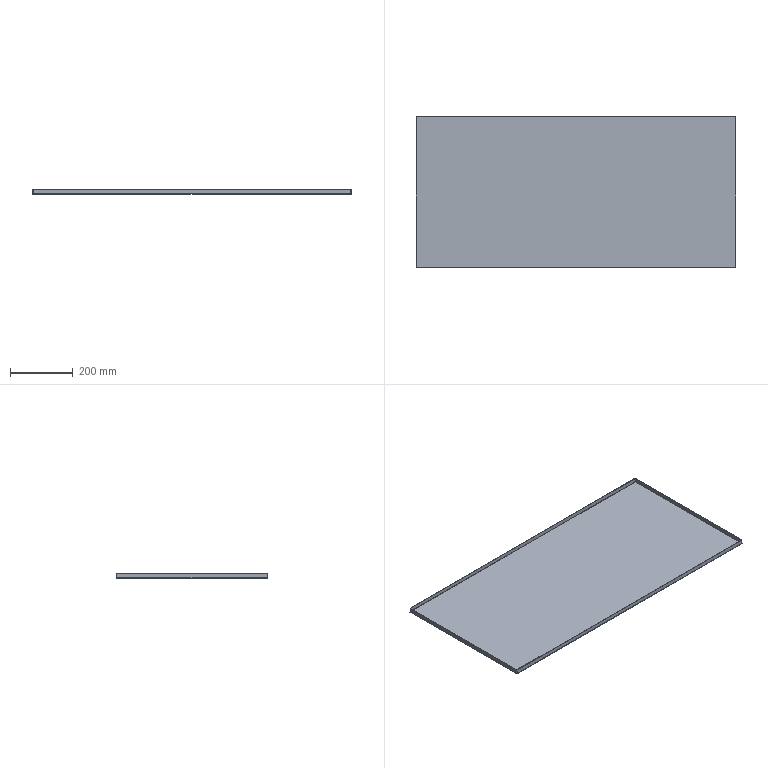Part | SolidWorks | 1 solid | 38 faces | box 1020 x 485 x 15 mm | volume 1064228 mm3 | plane 22 | spline 8 | cylinder 8 | commonest cylinder face diameters 0.2 x4 4.2 x4
STEP:
#1=CARTESIAN_POINT('',(507.9,-240.4,-2.));
#2=VERTEX_POINT('',#1);
#3=CARTESIAN_POINT('',(-507.9,-240.4,-2.));
#4=VERTEX_POINT('',#3);
#5=CARTESIAN_POINT('',(507.9,-240.4,-2.));
#6=DIRECTION('',(-1.,0.,0.));
#7=VECTOR('',#6,1000.);
#8=LINE('',#5,#7);
#9=EDGE_CURVE('',#2,#4,#8,.T.);
#10=ORIENTED_EDGE('',*,*,#9,.T.);
#11=CARTESIAN_POINT('',(-507.9,240.4,-2.));
#12=VERTEX_POINT('',#11);
#13=CARTESIAN_POINT('',(-507.9,-240.4,-2.));
#14=DIRECTION('',(0.,1.,0.));
#15=VECTOR('',#14,1000.);
#16=LINE('',#13,#15);
#17=EDGE_CURVE('',#4,#12,#16,.T.);
#18=ORIENTED_EDGE('',*,*,#17,.T.);
#19=CARTESIAN_POINT('',(507.9,240.4,-2.));
#20=VERTEX_POINT('',#19);
#21=CARTESIAN_POINT('',(-507.9,240.4,-2.));
#22=DIRECTION('',(1.,0.,0.));
#23=VECTOR('',#22,1000.);
#24=LINE('',#21,#23);
#25=EDGE_CURVE('',#12,#20,#24,.T.);
#26=ORIENTED_EDGE('',*,*,#25,.T.);
#27=CARTESIAN_POINT('',(507.9,240.4,-2.));
#28=DIRECTION('',(0.,-1.,0.));
#29=VECTOR('',#28,1000.);
#30=LINE('',#27,#29);
#31=EDGE_CURVE('',#20,#2,#30,.T.);
#32=ORIENTED_EDGE('',*,*,#31,.T.);
#33=EDGE_LOOP('',(#10,#18,#26,#32));
#34=FACE_OUTER_BOUND('',#33,.T.);
#35=CARTESIAN_POINT('',(0.,0.,-2.));
#36=DIRECTION('',(0.,0.,1.));
#37=DIRECTION('',(1.,0.,0.));
#38=AXIS2_PLACEMENT_3D('',#35,#36,#37);
#39=PLANE('',#38);
#40=ADVANCED_FACE('',(#34),#39,.F.);
#41=CARTESIAN_POINT('',(-507.9,-240.4,0.));
#42=VERTEX_POINT('',#41);
#43=CARTESIAN_POINT('',(-507.9,240.4,0.));
#44=VERTEX_POINT('',#43);
#45=CARTESIAN_POINT('',(-507.9,-240.4,0.));
#46=DIRECTION('',(0.,1.,0.));
#47=VECTOR('',#46,1000.);
#48=LINE('',#45,#47);
#49=EDGE_CURVE('',#42,#44,#48,.T.);
#50=ORIENTED_EDGE('',*,*,#49,.F.);
#51=CARTESIAN_POINT('',(507.9,-240.4,0.));
#52=VERTEX_POINT('',#51);
#53=CARTESIAN_POINT('',(507.9,-240.4,0.));
#54=DIRECTION('',(-1.,0.,0.));
#55=VECTOR('',#54,1000.);
#56=LINE('',#53,#55);
#57=EDGE_CURVE('',#52,#42,#56,.T.);
#58=ORIENTED_EDGE('',*,*,#57,.F.);
#59=CARTESIAN_POINT('',(507.9,240.4,0.));
#60=VERTEX_POINT('',#59);
#61=CARTESIAN_POINT('',(507.9,240.4,0.));
#62=DIRECTION('',(0.,-1.,0.));
#63=VECTOR('',#62,1000.);
#64=LINE('',#61,#63);
#65=EDGE_CURVE('',#60,#52,#64,.T.);
#66=ORIENTED_EDGE('',*,*,#65,.F.);
#67=CARTESIAN_POINT('',(-507.9,240.4,0.));
#68=DIRECTION('',(1.,0.,0.));
#69=VECTOR('',#68,1000.);
#70=LINE('',#67,#69);
#71=EDGE_CURVE('',#44,#60,#70,.T.);
#72=ORIENTED_EDGE('',*,*,#71,.F.);
#73=EDGE_LOOP('',(#50,#58,#66,#72));
#74=FACE_OUTER_BOUND('',#73,.T.);
#75=CARTESIAN_POINT('',(0.,0.,0.));
#76=DIRECTION('',(0.,0.,1.));
#77=DIRECTION('',(1.,0.,0.));
#78=AXIS2_PLACEMENT_3D('',#75,#76,#77);
#79=PLANE('',#78);
#80=ADVANCED_FACE('',(#74),#79,.T.);
#81=CARTESIAN_POINT('',(-510.,239.793,0.1));
#82=VERTEX_POINT('',#81);
#83=CARTESIAN_POINT('',(-508.,239.793,0.1));
#84=VERTEX_POINT('',#83);
#85=CARTESIAN_POINT('',(-508.,239.793,0.1));
#86=DIRECTION('',(1.,0.,0.));
#87=VECTOR('',#86,1000.);
#88=LINE('',#85,#87);
#89=EDGE_CURVE('',#82,#84,#88,.T.);
#90=ORIENTED_EDGE('',*,*,#89,.T.);
#91=CARTESIAN_POINT('',(-507.9,240.4,0.));
#92=CARTESIAN_POINT('',(-507.926,240.299,0.));
#93=CARTESIAN_POINT('',(-507.952,240.198,0.01078));
#94=CARTESIAN_POINT('',(-507.989,239.995,0.0478));
#95=CARTESIAN_POINT('',(-508.,239.894,0.07382));
#96=CARTESIAN_POINT('',(-508.,239.793,0.1));
#97=B_SPLINE_CURVE_WITH_KNOTS('',3,(#91,#92,#93,#94,#95,#96),.UNSPECIFIED.,.F.,.F.,(4,2,4),(0.,0.5,1.),.UNSPECIFIED.);
#98=EDGE_CURVE('',#44,#84,#97,.T.);
#99=ORIENTED_EDGE('',*,*,#98,.F.);
#100=CARTESIAN_POINT('',(-507.9,240.4,0.));
#101=DIRECTION('',(0.,0.,-1.));
#102=VECTOR('',#101,1000.);
#103=LINE('',#100,#102);
#104=EDGE_CURVE('',#44,#12,#103,.T.);
#105=ORIENTED_EDGE('',*,*,#104,.T.);
#106=CARTESIAN_POINT('',(-507.9,240.4,-2.));
#107=CARTESIAN_POINT('',(-508.039,240.374,-2.));
#108=CARTESIAN_POINT('',(-508.175,240.349,-1.986));
#109=CARTESIAN_POINT('',(-508.443,240.299,-1.933));
#110=CARTESIAN_POINT('',(-508.576,240.274,-1.893));
#111=CARTESIAN_POINT('',(-508.831,240.223,-1.787));
#112=CARTESIAN_POINT('',(-508.951,240.198,-1.723));
#113=CARTESIAN_POINT('',(-509.179,240.147,-1.571));
#114=CARTESIAN_POINT('',(-509.287,240.122,-1.482));
#115=CARTESIAN_POINT('',(-509.481,240.071,-1.289));
#116=CARTESIAN_POINT('',(-509.568,240.046,-1.183));
#117=CARTESIAN_POINT('',(-509.721,239.996,-0.9542));
#118=CARTESIAN_POINT('',(-509.787,239.97,-0.8315));
#119=CARTESIAN_POINT('',(-509.944,239.895,-0.4527));
#120=CARTESIAN_POINT('',(-510.,239.844,-0.1773));
#121=CARTESIAN_POINT('',(-510.,239.793,0.1));
#122=B_SPLINE_CURVE_WITH_KNOTS('',3,(#106,#107,#108,#109,#110,#111,#112,#113,#114,#115,#116,#117,#118,#119,#120,#121),.UNSPECIFIED.,.F.,.F.,(4,2,2,2,2,2,2,4),(0.,0.0004169,0.0008339,0.001251,0.001668,0.002085,0.002502,0.003336),.UNSPECIFIED.);
#123=EDGE_CURVE('',#12,#82,#122,.T.);
#124=ORIENTED_EDGE('',*,*,#123,.T.);
#125=EDGE_LOOP('',(#90,#99,#105,#124));
#126=FACE_OUTER_BOUND('',#125,.T.);
#127=CARTESIAN_POINT('',(-507.9,240.4,-2.02));
#128=CARTESIAN_POINT('',(-508.178,240.349,-2.02));
#129=CARTESIAN_POINT('',(-508.455,240.299,-1.965));
#130=CARTESIAN_POINT('',(-508.968,240.198,-1.752));
#131=CARTESIAN_POINT('',(-509.203,240.147,-1.595));
#132=CARTESIAN_POINT('',(-509.595,240.046,-1.203));
#133=CARTESIAN_POINT('',(-509.752,239.995,-0.9677));
#134=CARTESIAN_POINT('',(-509.965,239.894,-0.4549));
#135=CARTESIAN_POINT('',(-510.02,239.843,-0.1776));
#136=CARTESIAN_POINT('',(-510.02,239.793,0.1));
#137=CARTESIAN_POINT('',(-507.9,240.4,-2.));
#138=CARTESIAN_POINT('',(-508.175,240.349,-2.));
#139=CARTESIAN_POINT('',(-508.45,240.299,-1.945));
#140=CARTESIAN_POINT('',(-508.958,240.198,-1.735));
#141=CARTESIAN_POINT('',(-509.191,240.147,-1.579));
#142=CARTESIAN_POINT('',(-509.579,240.046,-1.191));
#143=CARTESIAN_POINT('',(-509.735,239.995,-0.9576));
#144=CARTESIAN_POINT('',(-509.945,239.894,-0.4497));
#145=CARTESIAN_POINT('',(-510.,239.843,-0.1749));
#146=CARTESIAN_POINT('',(-510.,239.793,0.1));
#147=CARTESIAN_POINT('',(-507.9,240.4,0.));
#148=CARTESIAN_POINT('',(-507.913,240.349,0.));
#149=CARTESIAN_POINT('',(-507.926,240.299,0.002603));
#150=CARTESIAN_POINT('',(-507.95,240.198,0.01262));
#151=CARTESIAN_POINT('',(-507.961,240.147,0.02003));
#152=CARTESIAN_POINT('',(-507.98,240.046,0.03855));
#153=CARTESIAN_POINT('',(-507.987,239.995,0.04964));
#154=CARTESIAN_POINT('',(-507.997,239.894,0.07383));
#155=CARTESIAN_POINT('',(-508.,239.843,0.08691));
#156=CARTESIAN_POINT('',(-508.,239.793,0.1));
#157=B_SPLINE_SURFACE_WITH_KNOTS('',1,3,((#127,#128,#129,#130,#131,#132,#133,#134,#135,#136),(#137,#138,#139,#140,#141,#142,#143,#144,#145,#146),(#147,#148,#149,#150,#151,#152,#153,#154,#155,#156)),.UNSPECIFIED.,.F.,.F.,.F.,(2,1,2),(4,2,2,2,4),(-0.01,0.,1.),(0.,0.25,0.5,0.75,1.),.UNSPECIFIED.);
#158=ADVANCED_FACE('',(#126),#157,.F.);
#159=CARTESIAN_POINT('',(-508.,-239.793,0.1));
#160=VERTEX_POINT('',#159);
#161=CARTESIAN_POINT('',(-508.,-239.793,0.1));
#162=CARTESIAN_POINT('',(-508.,-239.894,0.07382));
#163=CARTESIAN_POINT('',(-507.989,-239.995,0.0478));
#164=CARTESIAN_POINT('',(-507.952,-240.198,0.01078));
#165=CARTESIAN_POINT('',(-507.926,-240.299,0.));
#166=CARTESIAN_POINT('',(-507.9,-240.4,0.));
#167=B_SPLINE_CURVE_WITH_KNOTS('',3,(#161,#162,#163,#164,#165,#166),.UNSPECIFIED.,.F.,.F.,(4,2,4),(0.,0.5,1.),.UNSPECIFIED.);
#168=EDGE_CURVE('',#160,#42,#167,.T.);
#169=ORIENTED_EDGE('',*,*,#168,.F.);
#170=CARTESIAN_POINT('',(-510.,-239.793,0.1));
#171=VERTEX_POINT('',#170);
#172=CARTESIAN_POINT('',(-508.,-239.793,0.1));
#173=DIRECTION('',(1.,0.,0.));
#174=VECTOR('',#173,1000.);
#175=LINE('',#172,#174);
#176=EDGE_CURVE('',#171,#160,#175,.T.);
#177=ORIENTED_EDGE('',*,*,#176,.F.);
#178=CARTESIAN_POINT('',(-510.,-239.793,0.1));
#179=CARTESIAN_POINT('',(-510.,-239.818,-0.03865));
#180=CARTESIAN_POINT('',(-509.986,-239.844,-0.175));
#181=CARTESIAN_POINT('',(-509.933,-239.894,-0.4432));
#182=CARTESIAN_POINT('',(-509.893,-239.919,-0.5764));
#183=CARTESIAN_POINT('',(-509.787,-239.97,-0.8308));
#184=CARTESIAN_POINT('',(-509.723,-239.995,-0.9514));
#185=CARTESIAN_POINT('',(-509.571,-240.045,-1.179));
#186=CARTESIAN_POINT('',(-509.482,-240.071,-1.287));
#187=CARTESIAN_POINT('',(-509.289,-240.122,-1.481));
#188=CARTESIAN_POINT('',(-509.183,-240.147,-1.568));
#189=CARTESIAN_POINT('',(-508.954,-240.197,-1.721));
#190=CARTESIAN_POINT('',(-508.832,-240.223,-1.787));
#191=CARTESIAN_POINT('',(-508.453,-240.298,-1.944));
#192=CARTESIAN_POINT('',(-508.177,-240.349,-2.));
#193=CARTESIAN_POINT('',(-507.9,-240.4,-2.));
#194=B_SPLINE_CURVE_WITH_KNOTS('',3,(#178,#179,#180,#181,#182,#183,#184,#185,#186,#187,#188,#189,#190,#191,#192,#193),.UNSPECIFIED.,.F.,.F.,(4,2,2,2,2,2,2,4),(0.,0.0004169,0.0008339,0.001251,0.001668,0.002085,0.002502,0.003336),.UNSPECIFIED.);
#195=EDGE_CURVE('',#171,#4,#194,.T.);
#196=ORIENTED_EDGE('',*,*,#195,.T.);
#197=CARTESIAN_POINT('',(-507.9,-240.4,0.));
#198=DIRECTION('',(0.,0.,-1.));
#199=VECTOR('',#198,1000.);
#200=LINE('',#197,#199);
#201=EDGE_CURVE('',#42,#4,#200,.T.);
#202=ORIENTED_EDGE('',*,*,#201,.F.);
#203=EDGE_LOOP('',(#169,#177,#196,#202));
#204=FACE_OUTER_BOUND('',#203,.T.);
#205=CARTESIAN_POINT('',(-510.02,-239.793,0.1));
#206=CARTESIAN_POINT('',(-510.02,-239.843,-0.1776));
#207=CARTESIAN_POINT('',(-509.965,-239.894,-0.4549));
#208=CARTESIAN_POINT('',(-509.752,-239.995,-0.9677));
#209=CARTESIAN_POINT('',(-509.595,-240.046,-1.203));
#210=CARTESIAN_POINT('',(-509.203,-240.147,-1.595));
#211=CARTESIAN_POINT('',(-508.968,-240.198,-1.752));
#212=CARTESIAN_POINT('',(-508.455,-240.299,-1.965));
#213=CARTESIAN_POINT('',(-508.178,-240.349,-2.02));
#214=CARTESIAN_POINT('',(-507.9,-240.4,-2.02));
#215=CARTESIAN_POINT('',(-510.,-239.793,0.1));
#216=CARTESIAN_POINT('',(-510.,-239.843,-0.1749));
#217=CARTESIAN_POINT('',(-509.945,-239.894,-0.4497));
#218=CARTESIAN_POINT('',(-509.735,-239.995,-0.9576));
#219=CARTESIAN_POINT('',(-509.579,-240.046,-1.191));
#220=CARTESIAN_POINT('',(-509.191,-240.147,-1.579));
#221=CARTESIAN_POINT('',(-508.958,-240.198,-1.735));
#222=CARTESIAN_POINT('',(-508.45,-240.299,-1.945));
#223=CARTESIAN_POINT('',(-508.175,-240.349,-2.));
#224=CARTESIAN_POINT('',(-507.9,-240.4,-2.));
#225=CARTESIAN_POINT('',(-508.,-239.793,0.1));
#226=CARTESIAN_POINT('',(-508.,-239.843,0.08691));
#227=CARTESIAN_POINT('',(-507.997,-239.894,0.07383));
#228=CARTESIAN_POINT('',(-507.987,-239.995,0.04964));
#229=CARTESIAN_POINT('',(-507.98,-240.046,0.03855));
#230=CARTESIAN_POINT('',(-507.961,-240.147,0.02003));
#231=CARTESIAN_POINT('',(-507.95,-240.198,0.01262));
#232=CARTESIAN_POINT('',(-507.926,-240.299,0.002603));
#233=CARTESIAN_POINT('',(-507.913,-240.349,0.));
#234=CARTESIAN_POINT('',(-507.9,-240.4,0.));
#235=B_SPLINE_SURFACE_WITH_KNOTS('',1,3,((#205,#206,#207,#208,#209,#210,#211,#212,#213,#214),(#215,#216,#217,#218,#219,#220,#221,#222,#223,#224),(#225,#226,#227,#228,#229,#230,#231,#232,#233,#234)),.UNSPECIFIED.,.F.,.F.,.F.,(2,1,2),(4,2,2,2,4),(-0.01,0.,1.),(0.,0.25,0.5,0.75,1.),.UNSPECIFIED.);
#236=ADVANCED_FACE('',(#204),#235,.F.);
#237=ORIENTED_EDGE('',*,*,#17,.F.);
#238=ORIENTED_EDGE('',*,*,#195,.F.);
#239=CARTESIAN_POINT('',(-510.,242.5,0.1));
#240=DIRECTION('',(0.,1.,0.));
#241=VECTOR('',#240,1000.);
#242=LINE('',#239,#241);
#243=EDGE_CURVE('',#171,#82,#242,.T.);
#244=ORIENTED_EDGE('',*,*,#243,.T.);
#245=ORIENTED_EDGE('',*,*,#123,.F.);
#246=EDGE_LOOP('',(#237,#238,#244,#245));
#247=FACE_OUTER_BOUND('',#246,.T.);
#248=CARTESIAN_POINT('',(-507.9,-240.4,0.1));
#249=DIRECTION('',(0.,-1.,0.));
#250=DIRECTION('',(-1.,0.,0.));
#251=AXIS2_PLACEMENT_3D('',#248,#249,#250);
#252=CYLINDRICAL_SURFACE('',#251,2.1);
#253=ADVANCED_FACE('',(#247),#252,.T.);
#254=ORIENTED_EDGE('',*,*,#49,.T.);
#255=ORIENTED_EDGE('',*,*,#98,.T.);
#256=CARTESIAN_POINT('',(-508.,242.5,0.1));
#257=DIRECTION('',(0.,-1.,0.));
#258=VECTOR('',#257,1000.);
#259=LINE('',#256,#258);
#260=EDGE_CURVE('',#84,#160,#259,.T.);
#261=ORIENTED_EDGE('',*,*,#260,.T.);
#262=ORIENTED_EDGE('',*,*,#168,.T.);
#263=EDGE_LOOP('',(#254,#255,#261,#262));
#264=FACE_OUTER_BOUND('',#263,.T.);
#265=CARTESIAN_POINT('',(-507.9,-240.4,0.1));
#266=DIRECTION('',(0.,-1.,0.));
#267=DIRECTION('',(-1.,0.,0.));
#268=AXIS2_PLACEMENT_3D('',#265,#266,#267);
#269=CYLINDRICAL_SURFACE('',#268,0.1);
#270=ADVANCED_FACE('',(#264),#269,.F.);
#271=CARTESIAN_POINT('',(-510.,239.793,13.));
#272=VERTEX_POINT('',#271);
#273=CARTESIAN_POINT('',(-510.,239.793,0.));
#274=DIRECTION('',(0.,0.,1.));
#275=VECTOR('',#274,1000.);
#276=LINE('',#273,#275);
#277=EDGE_CURVE('',#82,#272,#276,.T.);
#278=ORIENTED_EDGE('',*,*,#277,.T.);
#279=CARTESIAN_POINT('',(-508.,239.793,13.));
#280=VERTEX_POINT('',#279);
#281=CARTESIAN_POINT('',(-508.,239.793,13.));
#282=DIRECTION('',(1.,0.,0.));
#283=VECTOR('',#282,1000.);
#284=LINE('',#281,#283);
#285=EDGE_CURVE('',#272,#280,#284,.T.);
#286=ORIENTED_EDGE('',*,*,#285,.T.);
#287=CARTESIAN_POINT('',(-508.,239.793,0.));
#288=DIRECTION('',(0.,0.,1.));
#289=VECTOR('',#288,1000.);
#290=LINE('',#287,#289);
#291=EDGE_CURVE('',#84,#280,#290,.T.);
#292=ORIENTED_EDGE('',*,*,#291,.F.);
#293=ORIENTED_EDGE('',*,*,#89,.F.);
#294=EDGE_LOOP('',(#278,#286,#292,#293));
#295=FACE_OUTER_BOUND('',#294,.T.);
#296=CARTESIAN_POINT('',(-508.,239.793,0.));
#297=DIRECTION('',(0.,1.,0.));
#298=DIRECTION('',(0.,0.,1.));
#299=AXIS2_PLACEMENT_3D('',#296,#297,#298);
#300=PLANE('',#299);
#301=ADVANCED_FACE('',(#295),#300,.T.);
#302=ORIENTED_EDGE('',*,*,#243,.F.);
#303=CARTESIAN_POINT('',(-510.,-239.793,13.));
#304=VERTEX_POINT('',#303);
#305=CARTESIAN_POINT('',(-510.,-239.793,0.));
#306=DIRECTION('',(0.,0.,1.));
#307=VECTOR('',#306,1000.);
#308=LINE('',#305,#307);
#309=EDGE_CURVE('',#171,#304,#308,.T.);
#310=ORIENTED_EDGE('',*,*,#309,.T.);
#311=CARTESIAN_POINT('',(-510.,0.,13.));
#312=DIRECTION('',(0.,1.,0.));
#313=VECTOR('',#312,1000.);
#314=LINE('',#311,#313);
#315=EDGE_CURVE('',#304,#272,#314,.T.);
#316=ORIENTED_EDGE('',*,*,#315,.T.);
#317=ORIENTED_EDGE('',*,*,#277,.F.);
#318=EDGE_LOOP('',(#302,#310,#316,#317));
#319=FACE_OUTER_BOUND('',#318,.T.);
#320=CARTESIAN_POINT('',(-510.,0.,0.));
#321=DIRECTION('',(1.,0.,0.));
#322=DIRECTION('',(0.,0.,-1.));
#323=AXIS2_PLACEMENT_3D('',#320,#321,#322);
#324=PLANE('',#323);
#325=ADVANCED_FACE('',(#319),#324,.F.);
#326=CARTESIAN_POINT('',(-508.,-239.793,13.));
#327=VERTEX_POINT('',#326);
#328=CARTESIAN_POINT('',(-508.,-239.793,0.));
#329=DIRECTION('',(0.,0.,1.));
#330=VECTOR('',#329,1000.);
#331=LINE('',#328,#330);
#332=EDGE_CURVE('',#160,#327,#331,.T.);
#333=ORIENTED_EDGE('',*,*,#332,.F.);
#334=ORIENTED_EDGE('',*,*,#260,.F.);
#335=ORIENTED_EDGE('',*,*,#291,.T.);
#336=CARTESIAN_POINT('',(-508.,242.5,13.));
#337=DIRECTION('',(0.,1.,0.));
#338=VECTOR('',#337,1000.);
#339=LINE('',#336,#338);
#340=EDGE_CURVE('',#327,#280,#339,.T.);
#341=ORIENTED_EDGE('',*,*,#340,.F.);
#342=EDGE_LOOP('',(#333,#334,#335,#341));
#343=FACE_OUTER_BOUND('',#342,.T.);
#344=CARTESIAN_POINT('',(-508.,0.,0.));
#345=DIRECTION('',(1.,0.,0.));
#346=DIRECTION('',(0.,0.,-1.));
#347=AXIS2_PLACEMENT_3D('',#344,#345,#346);
#348=PLANE('',#347);
#349=ADVANCED_FACE('',(#343),#348,.T.);
#350=ORIENTED_EDGE('',*,*,#315,.F.);
#351=CARTESIAN_POINT('',(-510.,-239.793,13.));
#352=DIRECTION('',(1.,0.,0.));
#353=VECTOR('',#352,1000.);
#354=LINE('',#351,#353);
#355=EDGE_CURVE('',#304,#327,#354,.T.);
#356=ORIENTED_EDGE('',*,*,#355,.T.);
#357=ORIENTED_EDGE('',*,*,#340,.T.);
#358=ORIENTED_EDGE('',*,*,#285,.F.);
#359=EDGE_LOOP('',(#350,#356,#357,#358));
#360=FACE_OUTER_BOUND('',#359,.T.);
#361=CARTESIAN_POINT('',(-510.,242.5,13.));
#362=DIRECTION('',(0.,0.,-1.));
#363=DIRECTION('',(-1.,0.,0.));
#364=AXIS2_PLACEMENT_3D('',#361,#362,#363);
#365=PLANE('',#364);
#366=ADVANCED_FACE('',(#360),#365,.F.);
#367=ORIENTED_EDGE('',*,*,#355,.F.);
#368=ORIENTED_EDGE('',*,*,#309,.F.);
#369=ORIENTED_EDGE('',*,*,#176,.T.);
#370=ORIENTED_EDGE('',*,*,#332,.T.);
#371=EDGE_LOOP('',(#367,#368,#369,#370));
#372=FACE_OUTER_BOUND('',#371,.T.);
#373=CARTESIAN_POINT('',(-508.,-239.793,0.));
#374=DIRECTION('',(0.,1.,0.));
#375=DIRECTION('',(0.,0.,1.));
#376=AXIS2_PLACEMENT_3D('',#373,#374,#375);
#377=PLANE('',#376);
#378=ADVANCED_FACE('',(#372),#377,.F.);
#379=CARTESIAN_POINT('',(507.293,242.5,0.1));
#380=VERTEX_POINT('',#379);
#381=CARTESIAN_POINT('',(507.293,240.5,0.1));
#382=VERTEX_POINT('',#381);
#383=CARTESIAN_POINT('',(507.293,240.5,0.1));
#384=DIRECTION('',(0.,-1.,0.));
#385=VECTOR('',#384,1000.);
#386=LINE('',#383,#385);
#387=EDGE_CURVE('',#380,#382,#386,.T.);
#388=ORIENTED_EDGE('',*,*,#387,.T.);
#389=CARTESIAN_POINT('',(507.9,240.4,0.));
#390=CARTESIAN_POINT('',(507.799,240.426,0.));
#391=CARTESIAN_POINT('',(507.698,240.452,0.01078));
#392=CARTESIAN_POINT('',(507.495,240.489,0.0478));
#393=CARTESIAN_POINT('',(507.394,240.5,0.07382));
#394=CARTESIAN_POINT('',(507.293,240.5,0.1));
#395=B_SPLINE_CURVE_WITH_KNOTS('',3,(#389,#390,#391,#392,#393,#394),.UNSPECIFIED.,.F.,.F.,(4,2,4),(0.,0.5,1.),.UNSPECIFIED.);
#396=EDGE_CURVE('',#60,#382,#395,.T.);
#397=ORIENTED_EDGE('',*,*,#396,.F.);
#398=CARTESIAN_POINT('',(507.9,240.4,0.));
#399=DIRECTION('',(0.,0.,-1.));
#400=VECTOR('',#399,1000.);
#401=LINE('',#398,#400);
#402=EDGE_CURVE('',#60,#20,#401,.T.);
#403=ORIENTED_EDGE('',*,*,#402,.T.);
#404=CARTESIAN_POINT('',(507.9,240.4,-2.));
#405=CARTESIAN_POINT('',(507.874,240.539,-2.));
#406=CARTESIAN_POINT('',(507.849,240.675,-1.986));
#407=CARTESIAN_POINT('',(507.799,240.943,-1.933));
#408=CARTESIAN_POINT('',(507.774,241.076,-1.893));
#409=CARTESIAN_POINT('',(507.723,241.331,-1.787));
#410=CARTESIAN_POINT('',(507.698,241.451,-1.723));
#411=CARTESIAN_POINT('',(507.647,241.679,-1.571));
#412=CARTESIAN_POINT('',(507.622,241.787,-1.482));
#413=CARTESIAN_POINT('',(507.571,241.981,-1.289));
#414=CARTESIAN_POINT('',(507.546,242.068,-1.183));
#415=CARTESIAN_POINT('',(507.496,242.221,-0.9542));
#416=CARTESIAN_POINT('',(507.47,242.287,-0.8315));
#417=CARTESIAN_POINT('',(507.395,242.444,-0.4527));
#418=CARTESIAN_POINT('',(507.344,242.5,-0.1773));
#419=CARTESIAN_POINT('',(507.293,242.5,0.1));
#420=B_SPLINE_CURVE_WITH_KNOTS('',3,(#404,#405,#406,#407,#408,#409,#410,#411,#412,#413,#414,#415,#416,#417,#418,#419),.UNSPECIFIED.,.F.,.F.,(4,2,2,2,2,2,2,4),(0.,0.0004169,0.0008339,0.001251,0.001668,0.002085,0.002502,0.003336),.UNSPECIFIED.);
#421=EDGE_CURVE('',#20,#380,#420,.T.);
#422=ORIENTED_EDGE('',*,*,#421,.T.);
#423=EDGE_LOOP('',(#388,#397,#403,#422));
#424=FACE_OUTER_BOUND('',#423,.T.);
#425=CARTESIAN_POINT('',(507.9,240.4,-2.02));
#426=CARTESIAN_POINT('',(507.849,240.678,-2.02));
#427=CARTESIAN_POINT('',(507.799,240.955,-1.965));
#428=CARTESIAN_POINT('',(507.698,241.468,-1.752));
#429=CARTESIAN_POINT('',(507.647,241.703,-1.595));
#430=CARTESIAN_POINT('',(507.546,242.095,-1.203));
#431=CARTESIAN_POINT('',(507.495,242.252,-0.9677));
#432=CARTESIAN_POINT('',(507.394,242.465,-0.4549));
#433=CARTESIAN_POINT('',(507.343,242.52,-0.1776));
#434=CARTESIAN_POINT('',(507.293,242.52,0.1));
#435=CARTESIAN_POINT('',(507.9,240.4,-2.));
#436=CARTESIAN_POINT('',(507.849,240.675,-2.));
#437=CARTESIAN_POINT('',(507.799,240.95,-1.945));
#438=CARTESIAN_POINT('',(507.698,241.458,-1.735));
#439=CARTESIAN_POINT('',(507.647,241.691,-1.579));
#440=CARTESIAN_POINT('',(507.546,242.079,-1.191));
#441=CARTESIAN_POINT('',(507.495,242.235,-0.9576));
#442=CARTESIAN_POINT('',(507.394,242.445,-0.4497));
#443=CARTESIAN_POINT('',(507.343,242.5,-0.1749));
#444=CARTESIAN_POINT('',(507.293,242.5,0.1));
#445=CARTESIAN_POINT('',(507.9,240.4,0.));
#446=CARTESIAN_POINT('',(507.849,240.413,0.));
#447=CARTESIAN_POINT('',(507.799,240.426,0.002603));
#448=CARTESIAN_POINT('',(507.698,240.45,0.01262));
#449=CARTESIAN_POINT('',(507.647,240.461,0.02003));
#450=CARTESIAN_POINT('',(507.546,240.48,0.03855));
#451=CARTESIAN_POINT('',(507.495,240.487,0.04964));
#452=CARTESIAN_POINT('',(507.394,240.497,0.07383));
#453=CARTESIAN_POINT('',(507.343,240.5,0.08691));
#454=CARTESIAN_POINT('',(507.293,240.5,0.1));
#455=B_SPLINE_SURFACE_WITH_KNOTS('',1,3,((#425,#426,#427,#428,#429,#430,#431,#432,#433,#434),(#435,#436,#437,#438,#439,#440,#441,#442,#443,#444),(#445,#446,#447,#448,#449,#450,#451,#452,#453,#454)),.UNSPECIFIED.,.F.,.F.,.F.,(2,1,2),(4,2,2,2,4),(-0.01,0.,1.),(0.,0.25,0.5,0.75,1.),.UNSPECIFIED.);
#456=ADVANCED_FACE('',(#424),#455,.F.);
#457=CARTESIAN_POINT('',(-507.293,240.5,0.1));
#458=VERTEX_POINT('',#457);
#459=CARTESIAN_POINT('',(-507.293,240.5,0.1));
#460=CARTESIAN_POINT('',(-507.394,240.5,0.07382));
#461=CARTESIAN_POINT('',(-507.495,240.489,0.0478));
#462=CARTESIAN_POINT('',(-507.698,240.452,0.01078));
#463=CARTESIAN_POINT('',(-507.799,240.426,0.));
#464=CARTESIAN_POINT('',(-507.9,240.4,0.));
#465=B_SPLINE_CURVE_WITH_KNOTS('',3,(#459,#460,#461,#462,#463,#464),.UNSPECIFIED.,.F.,.F.,(4,2,4),(0.,0.5,1.),.UNSPECIFIED.);
#466=EDGE_CURVE('',#458,#44,#465,.T.);
#467=ORIENTED_EDGE('',*,*,#466,.F.);
#468=CARTESIAN_POINT('',(-507.293,242.5,0.1));
#469=VERTEX_POINT('',#468);
#470=CARTESIAN_POINT('',(-507.293,240.5,0.1));
#471=DIRECTION('',(0.,-1.,0.));
#472=VECTOR('',#471,1000.);
#473=LINE('',#470,#472);
#474=EDGE_CURVE('',#469,#458,#473,.T.);
#475=ORIENTED_EDGE('',*,*,#474,.F.);
#476=CARTESIAN_POINT('',(-507.293,242.5,0.1));
#477=CARTESIAN_POINT('',(-507.318,242.5,-0.03865));
#478=CARTESIAN_POINT('',(-507.344,242.486,-0.175));
#479=CARTESIAN_POINT('',(-507.394,242.433,-0.4432));
#480=CARTESIAN_POINT('',(-507.419,242.393,-0.5764));
#481=CARTESIAN_POINT('',(-507.47,242.287,-0.8308));
#482=CARTESIAN_POINT('',(-507.495,242.223,-0.9514));
#483=CARTESIAN_POINT('',(-507.545,242.071,-1.179));
#484=CARTESIAN_POINT('',(-507.571,241.982,-1.287));
#485=CARTESIAN_POINT('',(-507.622,241.789,-1.481));
#486=CARTESIAN_POINT('',(-507.647,241.683,-1.568));
#487=CARTESIAN_POINT('',(-507.697,241.454,-1.721));
#488=CARTESIAN_POINT('',(-507.723,241.332,-1.787));
#489=CARTESIAN_POINT('',(-507.798,240.953,-1.944));
#490=CARTESIAN_POINT('',(-507.849,240.677,-2.));
#491=CARTESIAN_POINT('',(-507.9,240.4,-2.));
#492=B_SPLINE_CURVE_WITH_KNOTS('',3,(#476,#477,#478,#479,#480,#481,#482,#483,#484,#485,#486,#487,#488,#489,#490,#491),.UNSPECIFIED.,.F.,.F.,(4,2,2,2,2,2,2,4),(0.,0.0004169,0.0008339,0.001251,0.001668,0.002085,0.002502,0.003336),.UNSPECIFIED.);
#493=EDGE_CURVE('',#469,#12,#492,.T.);
#494=ORIENTED_EDGE('',*,*,#493,.T.);
#495=ORIENTED_EDGE('',*,*,#104,.F.);
#496=EDGE_LOOP('',(#467,#475,#494,#495));
#497=FACE_OUTER_BOUND('',#496,.T.);
#498=CARTESIAN_POINT('',(-507.293,242.52,0.1));
#499=CARTESIAN_POINT('',(-507.343,242.52,-0.1776));
#500=CARTESIAN_POINT('',(-507.394,242.465,-0.4549));
#501=CARTESIAN_POINT('',(-507.495,242.252,-0.9677));
#502=CARTESIAN_POINT('',(-507.546,242.095,-1.203));
#503=CARTESIAN_POINT('',(-507.647,241.703,-1.595));
#504=CARTESIAN_POINT('',(-507.698,241.468,-1.752));
#505=CARTESIAN_POINT('',(-507.799,240.955,-1.965));
#506=CARTESIAN_POINT('',(-507.849,240.678,-2.02));
#507=CARTESIAN_POINT('',(-507.9,240.4,-2.02));
#508=CARTESIAN_POINT('',(-507.293,242.5,0.1));
#509=CARTESIAN_POINT('',(-507.343,242.5,-0.1749));
#510=CARTESIAN_POINT('',(-507.394,242.445,-0.4497));
#511=CARTESIAN_POINT('',(-507.495,242.235,-0.9576));
#512=CARTESIAN_POINT('',(-507.546,242.079,-1.191));
#513=CARTESIAN_POINT('',(-507.647,241.691,-1.579));
#514=CARTESIAN_POINT('',(-507.698,241.458,-1.735));
#515=CARTESIAN_POINT('',(-507.799,240.95,-1.945));
#516=CARTESIAN_POINT('',(-507.849,240.675,-2.));
#517=CARTESIAN_POINT('',(-507.9,240.4,-2.));
#518=CARTESIAN_POINT('',(-507.293,240.5,0.1));
#519=CARTESIAN_POINT('',(-507.343,240.5,0.08691));
#520=CARTESIAN_POINT('',(-507.394,240.497,0.07383));
#521=CARTESIAN_POINT('',(-507.495,240.487,0.04964));
#522=CARTESIAN_POINT('',(-507.546,240.48,0.03855));
#523=CARTESIAN_POINT('',(-507.647,240.461,0.02003));
#524=CARTESIAN_POINT('',(-507.698,240.45,0.01262));
#525=CARTESIAN_POINT('',(-507.799,240.426,0.002603));
#526=CARTESIAN_POINT('',(-507.849,240.413,0.));
#527=CARTESIAN_POINT('',(-507.9,240.4,0.));
#528=B_SPLINE_SURFACE_WITH_KNOTS('',1,3,((#498,#499,#500,#501,#502,#503,#504,#505,#506,#507),(#508,#509,#510,#511,#512,#513,#514,#515,#516,#517),(#518,#519,#520,#521,#522,#523,#524,#525,#526,#527)),.UNSPECIFIED.,.F.,.F.,.F.,(2,1,2),(4,2,2,2,4),(-0.01,0.,1.),(0.,0.25,0.5,0.75,1.),.UNSPECIFIED.);
#529=ADVANCED_FACE('',(#497),#528,.F.);
#530=ORIENTED_EDGE('',*,*,#25,.F.);
#531=ORIENTED_EDGE('',*,*,#493,.F.);
#532=CARTESIAN_POINT('',(510.,242.5,0.1));
#533=DIRECTION('',(1.,0.,0.));
#534=VECTOR('',#533,1000.);
#535=LINE('',#532,#534);
#536=EDGE_CURVE('',#469,#380,#535,.T.);
#537=ORIENTED_EDGE('',*,*,#536,.T.);
#538=ORIENTED_EDGE('',*,*,#421,.F.);
#539=EDGE_LOOP('',(#530,#531,#537,#538));
#540=FACE_OUTER_BOUND('',#539,.T.);
#541=CARTESIAN_POINT('',(-507.9,240.4,0.1));
#542=DIRECTION('',(-1.,0.,0.));
#543=DIRECTION('',(0.,1.,0.));
#544=AXIS2_PLACEMENT_3D('',#541,#542,#543);
#545=CYLINDRICAL_SURFACE('',#544,2.1);
#546=ADVANCED_FACE('',(#540),#545,.T.);
#547=ORIENTED_EDGE('',*,*,#71,.T.);
#548=ORIENTED_EDGE('',*,*,#396,.T.);
#549=CARTESIAN_POINT('',(510.,240.5,0.1));
#550=DIRECTION('',(-1.,0.,0.));
#551=VECTOR('',#550,1000.);
#552=LINE('',#549,#551);
#553=EDGE_CURVE('',#382,#458,#552,.T.);
#554=ORIENTED_EDGE('',*,*,#553,.T.);
#555=ORIENTED_EDGE('',*,*,#466,.T.);
#556=EDGE_LOOP('',(#547,#548,#554,#555));
#557=FACE_OUTER_BOUND('',#556,.T.);
#558=CARTESIAN_POINT('',(-507.9,240.4,0.1));
#559=DIRECTION('',(-1.,0.,0.));
#560=DIRECTION('',(0.,1.,0.));
#561=AXIS2_PLACEMENT_3D('',#558,#559,#560);
#562=CYLINDRICAL_SURFACE('',#561,0.1);
#563=ADVANCED_FACE('',(#557),#562,.F.);
#564=CARTESIAN_POINT('',(507.293,242.5,13.));
#565=VERTEX_POINT('',#564);
#566=CARTESIAN_POINT('',(507.293,242.5,0.));
#567=DIRECTION('',(0.,0.,1.));
#568=VECTOR('',#567,1000.);
#569=LINE('',#566,#568);
#570=EDGE_CURVE('',#380,#565,#569,.T.);
#571=ORIENTED_EDGE('',*,*,#570,.T.);
#572=CARTESIAN_POINT('',(507.293,240.5,13.));
#573=VERTEX_POINT('',#572);
#574=CARTESIAN_POINT('',(507.293,240.5,13.));
#575=DIRECTION('',(0.,-1.,0.));
#576=VECTOR('',#575,1000.);
#577=LINE('',#574,#576);
#578=EDGE_CURVE('',#565,#573,#577,.T.);
#579=ORIENTED_EDGE('',*,*,#578,.T.);
#580=CARTESIAN_POINT('',(507.293,240.5,0.));
#581=DIRECTION('',(0.,0.,1.));
#582=VECTOR('',#581,1000.);
#583=LINE('',#580,#582);
#584=EDGE_CURVE('',#382,#573,#583,.T.);
#585=ORIENTED_EDGE('',*,*,#584,.F.);
#586=ORIENTED_EDGE('',*,*,#387,.F.);
#587=EDGE_LOOP('',(#571,#579,#585,#586));
#588=FACE_OUTER_BOUND('',#587,.T.);
#589=CARTESIAN_POINT('',(507.293,240.5,0.));
#590=DIRECTION('',(1.,0.,0.));
#591=DIRECTION('',(0.,0.,-1.));
#592=AXIS2_PLACEMENT_3D('',#589,#590,#591);
#593=PLANE('',#592);
#594=ADVANCED_FACE('',(#588),#593,.T.);
#595=ORIENTED_EDGE('',*,*,#536,.F.);
#596=CARTESIAN_POINT('',(-507.293,242.5,13.));
#597=VERTEX_POINT('',#596);
#598=CARTESIAN_POINT('',(-507.293,242.5,0.));
#599=DIRECTION('',(0.,0.,1.));
#600=VECTOR('',#599,1000.);
#601=LINE('',#598,#600);
#602=EDGE_CURVE('',#469,#597,#601,.T.);
#603=ORIENTED_EDGE('',*,*,#602,.T.);
#604=CARTESIAN_POINT('',(0.,242.5,13.));
#605=DIRECTION('',(1.,0.,0.));
#606=VECTOR('',#605,1000.);
#607=LINE('',#604,#606);
#608=EDGE_CURVE('',#597,#565,#607,.T.);
#609=ORIENTED_EDGE('',*,*,#608,.T.);
#610=ORIENTED_EDGE('',*,*,#570,.F.);
#611=EDGE_LOOP('',(#595,#603,#609,#610));
#612=FACE_OUTER_BOUND('',#611,.T.);
#613=CARTESIAN_POINT('',(0.,242.5,0.));
#614=DIRECTION('',(0.,-1.,0.));
#615=DIRECTION('',(0.,0.,-1.));
#616=AXIS2_PLACEMENT_3D('',#613,#614,#615);
#617=PLANE('',#616);
#618=ADVANCED_FACE('',(#612),#617,.F.);
#619=CARTESIAN_POINT('',(-507.293,240.5,13.));
#620=VERTEX_POINT('',#619);
#621=CARTESIAN_POINT('',(-507.293,240.5,0.));
#622=DIRECTION('',(0.,0.,1.));
#623=VECTOR('',#622,1000.);
#624=LINE('',#621,#623);
#625=EDGE_CURVE('',#458,#620,#624,.T.);
#626=ORIENTED_EDGE('',*,*,#625,.F.);
#627=ORIENTED_EDGE('',*,*,#553,.F.);
#628=ORIENTED_EDGE('',*,*,#584,.T.);
#629=CARTESIAN_POINT('',(510.,240.5,13.));
#630=DIRECTION('',(1.,0.,0.));
#631=VECTOR('',#630,1000.);
#632=LINE('',#629,#631);
#633=EDGE_CURVE('',#620,#573,#632,.T.);
#634=ORIENTED_EDGE('',*,*,#633,.F.);
#635=EDGE_LOOP('',(#626,#627,#628,#634));
#636=FACE_OUTER_BOUND('',#635,.T.);
#637=CARTESIAN_POINT('',(0.,240.5,0.));
#638=DIRECTION('',(0.,-1.,0.));
#639=DIRECTION('',(0.,0.,-1.));
#640=AXIS2_PLACEMENT_3D('',#637,#638,#639);
#641=PLANE('',#640);
#642=ADVANCED_FACE('',(#636),#641,.T.);
#643=ORIENTED_EDGE('',*,*,#608,.F.);
#644=CARTESIAN_POINT('',(-507.293,242.5,13.));
#645=DIRECTION('',(0.,-1.,0.));
#646=VECTOR('',#645,1000.);
#647=LINE('',#644,#646);
#648=EDGE_CURVE('',#597,#620,#647,.T.);
#649=ORIENTED_EDGE('',*,*,#648,.T.);
#650=ORIENTED_EDGE('',*,*,#633,.T.);
#651=ORIENTED_EDGE('',*,*,#578,.F.);
#652=EDGE_LOOP('',(#643,#649,#650,#651));
#653=FACE_OUTER_BOUND('',#652,.T.);
#654=CARTESIAN_POINT('',(510.,242.5,13.));
#655=DIRECTION('',(0.,0.,-1.));
#656=DIRECTION('',(0.,1.,0.));
#657=AXIS2_PLACEMENT_3D('',#654,#655,#656);
#658=PLANE('',#657);
#659=ADVANCED_FACE('',(#653),#658,.F.);
#660=ORIENTED_EDGE('',*,*,#648,.F.);
#661=ORIENTED_EDGE('',*,*,#602,.F.);
#662=ORIENTED_EDGE('',*,*,#474,.T.);
#663=ORIENTED_EDGE('',*,*,#625,.T.);
#664=EDGE_LOOP('',(#660,#661,#662,#663));
#665=FACE_OUTER_BOUND('',#664,.T.);
#666=CARTESIAN_POINT('',(-507.293,240.5,0.));
#667=DIRECTION('',(1.,0.,0.));
#668=DIRECTION('',(0.,0.,-1.));
#669=AXIS2_PLACEMENT_3D('',#666,#667,#668);
#670=PLANE('',#669);
#671=ADVANCED_FACE('',(#665),#670,.F.);
#672=CARTESIAN_POINT('',(510.,-239.793,0.1));
#673=VERTEX_POINT('',#672);
#674=CARTESIAN_POINT('',(508.,-239.793,0.1));
#675=VERTEX_POINT('',#674);
#676=CARTESIAN_POINT('',(508.,-239.793,0.1));
#677=DIRECTION('',(-1.,0.,0.));
#678=VECTOR('',#677,1000.);
#679=LINE('',#676,#678);
#680=EDGE_CURVE('',#673,#675,#679,.T.);
#681=ORIENTED_EDGE('',*,*,#680,.T.);
#682=CARTESIAN_POINT('',(507.9,-240.4,0.));
#683=CARTESIAN_POINT('',(507.926,-240.299,0.));
#684=CARTESIAN_POINT('',(507.952,-240.198,0.01078));
#685=CARTESIAN_POINT('',(507.989,-239.995,0.0478));
#686=CARTESIAN_POINT('',(508.,-239.894,0.07382));
#687=CARTESIAN_POINT('',(508.,-239.793,0.1));
#688=B_SPLINE_CURVE_WITH_KNOTS('',3,(#682,#683,#684,#685,#686,#687),.UNSPECIFIED.,.F.,.F.,(4,2,4),(0.,0.5,1.),.UNSPECIFIED.);
#689=EDGE_CURVE('',#52,#675,#688,.T.);
#690=ORIENTED_EDGE('',*,*,#689,.F.);
#691=CARTESIAN_POINT('',(507.9,-240.4,0.));
#692=DIRECTION('',(0.,0.,-1.));
#693=VECTOR('',#692,1000.);
#694=LINE('',#691,#693);
#695=EDGE_CURVE('',#52,#2,#694,.T.);
#696=ORIENTED_EDGE('',*,*,#695,.T.);
#697=CARTESIAN_POINT('',(507.9,-240.4,-2.));
#698=CARTESIAN_POINT('',(508.039,-240.374,-2.));
#699=CARTESIAN_POINT('',(508.175,-240.349,-1.986));
#700=CARTESIAN_POINT('',(508.443,-240.299,-1.933));
#701=CARTESIAN_POINT('',(508.576,-240.274,-1.893));
#702=CARTESIAN_POINT('',(508.831,-240.223,-1.787));
#703=CARTESIAN_POINT('',(508.951,-240.198,-1.723));
#704=CARTESIAN_POINT('',(509.179,-240.147,-1.571));
#705=CARTESIAN_POINT('',(509.287,-240.122,-1.482));
#706=CARTESIAN_POINT('',(509.481,-240.071,-1.289));
#707=CARTESIAN_POINT('',(509.568,-240.046,-1.183));
#708=CARTESIAN_POINT('',(509.721,-239.996,-0.9542));
#709=CARTESIAN_POINT('',(509.787,-239.97,-0.8315));
#710=CARTESIAN_POINT('',(509.944,-239.895,-0.4527));
#711=CARTESIAN_POINT('',(510.,-239.844,-0.1773));
#712=CARTESIAN_POINT('',(510.,-239.793,0.1));
#713=B_SPLINE_CURVE_WITH_KNOTS('',3,(#697,#698,#699,#700,#701,#702,#703,#704,#705,#706,#707,#708,#709,#710,#711,#712),.UNSPECIFIED.,.F.,.F.,(4,2,2,2,2,2,2,4),(0.,0.0004169,0.0008339,0.001251,0.001668,0.002085,0.002502,0.003336),.UNSPECIFIED.);
#714=EDGE_CURVE('',#2,#673,#713,.T.);
#715=ORIENTED_EDGE('',*,*,#714,.T.);
#716=EDGE_LOOP('',(#681,#690,#696,#715));
#717=FACE_OUTER_BOUND('',#716,.T.);
#718=CARTESIAN_POINT('',(507.9,-240.4,-2.02));
#719=CARTESIAN_POINT('',(508.178,-240.349,-2.02));
#720=CARTESIAN_POINT('',(508.455,-240.299,-1.965));
#721=CARTESIAN_POINT('',(508.968,-240.198,-1.752));
#722=CARTESIAN_POINT('',(509.203,-240.147,-1.595));
#723=CARTESIAN_POINT('',(509.595,-240.046,-1.203));
#724=CARTESIAN_POINT('',(509.752,-239.995,-0.9677));
#725=CARTESIAN_POINT('',(509.965,-239.894,-0.4549));
#726=CARTESIAN_POINT('',(510.02,-239.843,-0.1776));
#727=CARTESIAN_POINT('',(510.02,-239.793,0.1));
#728=CARTESIAN_POINT('',(507.9,-240.4,-2.));
#729=CARTESIAN_POINT('',(508.175,-240.349,-2.));
#730=CARTESIAN_POINT('',(508.45,-240.299,-1.945));
#731=CARTESIAN_POINT('',(508.958,-240.198,-1.735));
#732=CARTESIAN_POINT('',(509.191,-240.147,-1.579));
#733=CARTESIAN_POINT('',(509.579,-240.046,-1.191));
#734=CARTESIAN_POINT('',(509.735,-239.995,-0.9576));
#735=CARTESIAN_POINT('',(509.945,-239.894,-0.4497));
#736=CARTESIAN_POINT('',(510.,-239.843,-0.1749));
#737=CARTESIAN_POINT('',(510.,-239.793,0.1));
#738=CARTESIAN_POINT('',(507.9,-240.4,0.));
#739=CARTESIAN_POINT('',(507.913,-240.349,0.));
#740=CARTESIAN_POINT('',(507.926,-240.299,0.002603));
#741=CARTESIAN_POINT('',(507.95,-240.198,0.01262));
#742=CARTESIAN_POINT('',(507.961,-240.147,0.02003));
#743=CARTESIAN_POINT('',(507.98,-240.046,0.03855));
#744=CARTESIAN_POINT('',(507.987,-239.995,0.04964));
#745=CARTESIAN_POINT('',(507.997,-239.894,0.07383));
#746=CARTESIAN_POINT('',(508.,-239.843,0.08691));
#747=CARTESIAN_POINT('',(508.,-239.793,0.1));
#748=B_SPLINE_SURFACE_WITH_KNOTS('',1,3,((#718,#719,#720,#721,#722,#723,#724,#725,#726,#727),(#728,#729,#730,#731,#732,#733,#734,#735,#736,#737),(#738,#739,#740,#741,#742,#743,#744,#745,#746,#747)),.UNSPECIFIED.,.F.,.F.,.F.,(2,1,2),(4,2,2,2,4),(-0.01,0.,1.),(0.,0.25,0.5,0.75,1.),.UNSPECIFIED.);
#749=ADVANCED_FACE('',(#717),#748,.F.);
#750=CARTESIAN_POINT('',(508.,239.793,0.1));
#751=VERTEX_POINT('',#750);
#752=CARTESIAN_POINT('',(508.,239.793,0.1));
#753=CARTESIAN_POINT('',(508.,239.894,0.07382));
#754=CARTESIAN_POINT('',(507.989,239.995,0.0478));
#755=CARTESIAN_POINT('',(507.952,240.198,0.01078));
#756=CARTESIAN_POINT('',(507.926,240.299,0.));
#757=CARTESIAN_POINT('',(507.9,240.4,0.));
#758=B_SPLINE_CURVE_WITH_KNOTS('',3,(#752,#753,#754,#755,#756,#757),.UNSPECIFIED.,.F.,.F.,(4,2,4),(0.,0.5,1.),.UNSPECIFIED.);
#759=EDGE_CURVE('',#751,#60,#758,.T.);
#760=ORIENTED_EDGE('',*,*,#759,.F.);
#761=CARTESIAN_POINT('',(510.,239.793,0.1));
#762=VERTEX_POINT('',#761);
#763=CARTESIAN_POINT('',(508.,239.793,0.1));
#764=DIRECTION('',(-1.,0.,0.));
#765=VECTOR('',#764,1000.);
#766=LINE('',#763,#765);
#767=EDGE_CURVE('',#762,#751,#766,.T.);
#768=ORIENTED_EDGE('',*,*,#767,.F.);
#769=CARTESIAN_POINT('',(510.,239.793,0.1));
#770=CARTESIAN_POINT('',(510.,239.818,-0.03865));
#771=CARTESIAN_POINT('',(509.986,239.844,-0.175));
#772=CARTESIAN_POINT('',(509.933,239.894,-0.4432));
#773=CARTESIAN_POINT('',(509.893,239.919,-0.5764));
#774=CARTESIAN_POINT('',(509.787,239.97,-0.8308));
#775=CARTESIAN_POINT('',(509.723,239.995,-0.9514));
#776=CARTESIAN_POINT('',(509.571,240.045,-1.179));
#777=CARTESIAN_POINT('',(509.482,240.071,-1.287));
#778=CARTESIAN_POINT('',(509.289,240.122,-1.481));
#779=CARTESIAN_POINT('',(509.183,240.147,-1.568));
#780=CARTESIAN_POINT('',(508.954,240.197,-1.721));
#781=CARTESIAN_POINT('',(508.832,240.223,-1.787));
#782=CARTESIAN_POINT('',(508.453,240.298,-1.944));
#783=CARTESIAN_POINT('',(508.177,240.349,-2.));
#784=CARTESIAN_POINT('',(507.9,240.4,-2.));
#785=B_SPLINE_CURVE_WITH_KNOTS('',3,(#769,#770,#771,#772,#773,#774,#775,#776,#777,#778,#779,#780,#781,#782,#783,#784),.UNSPECIFIED.,.F.,.F.,(4,2,2,2,2,2,2,4),(0.,0.0004169,0.0008339,0.001251,0.001668,0.002085,0.002502,0.003336),.UNSPECIFIED.);
#786=EDGE_CURVE('',#762,#20,#785,.T.);
#787=ORIENTED_EDGE('',*,*,#786,.T.);
#788=ORIENTED_EDGE('',*,*,#402,.F.);
#789=EDGE_LOOP('',(#760,#768,#787,#788));
#790=FACE_OUTER_BOUND('',#789,.T.);
#791=CARTESIAN_POINT('',(510.02,239.793,0.1));
#792=CARTESIAN_POINT('',(510.02,239.843,-0.1776));
#793=CARTESIAN_POINT('',(509.965,239.894,-0.4549));
#794=CARTESIAN_POINT('',(509.752,239.995,-0.9677));
#795=CARTESIAN_POINT('',(509.595,240.046,-1.203));
#796=CARTESIAN_POINT('',(509.203,240.147,-1.595));
#797=CARTESIAN_POINT('',(508.968,240.198,-1.752));
#798=CARTESIAN_POINT('',(508.455,240.299,-1.965));
#799=CARTESIAN_POINT('',(508.178,240.349,-2.02));
#800=CARTESIAN_POINT('',(507.9,240.4,-2.02));
#801=CARTESIAN_POINT('',(510.,239.793,0.1));
#802=CARTESIAN_POINT('',(510.,239.843,-0.1749));
#803=CARTESIAN_POINT('',(509.945,239.894,-0.4497));
#804=CARTESIAN_POINT('',(509.735,239.995,-0.9576));
#805=CARTESIAN_POINT('',(509.579,240.046,-1.191));
#806=CARTESIAN_POINT('',(509.191,240.147,-1.579));
#807=CARTESIAN_POINT('',(508.958,240.198,-1.735));
#808=CARTESIAN_POINT('',(508.45,240.299,-1.945));
#809=CARTESIAN_POINT('',(508.175,240.349,-2.));
#810=CARTESIAN_POINT('',(507.9,240.4,-2.));
#811=CARTESIAN_POINT('',(508.,239.793,0.1));
#812=CARTESIAN_POINT('',(508.,239.843,0.08691));
#813=CARTESIAN_POINT('',(507.997,239.894,0.07383));
#814=CARTESIAN_POINT('',(507.987,239.995,0.04964));
#815=CARTESIAN_POINT('',(507.98,240.046,0.03855));
#816=CARTESIAN_POINT('',(507.961,240.147,0.02003));
#817=CARTESIAN_POINT('',(507.95,240.198,0.01262));
#818=CARTESIAN_POINT('',(507.926,240.299,0.002603));
#819=CARTESIAN_POINT('',(507.913,240.349,0.));
#820=CARTESIAN_POINT('',(507.9,240.4,0.));
#821=B_SPLINE_SURFACE_WITH_KNOTS('',1,3,((#791,#792,#793,#794,#795,#796,#797,#798,#799,#800),(#801,#802,#803,#804,#805,#806,#807,#808,#809,#810),(#811,#812,#813,#814,#815,#816,#817,#818,#819,#820)),.UNSPECIFIED.,.F.,.F.,.F.,(2,1,2),(4,2,2,2,4),(-0.01,0.,1.),(0.,0.25,0.5,0.75,1.),.UNSPECIFIED.);
#822=ADVANCED_FACE('',(#790),#821,.F.);
#823=ORIENTED_EDGE('',*,*,#31,.F.);
#824=ORIENTED_EDGE('',*,*,#786,.F.);
#825=CARTESIAN_POINT('',(510.,-242.5,0.1));
#826=DIRECTION('',(0.,-1.,0.));
#827=VECTOR('',#826,1000.);
#828=LINE('',#825,#827);
#829=EDGE_CURVE('',#762,#673,#828,.T.);
#830=ORIENTED_EDGE('',*,*,#829,.T.);
#831=ORIENTED_EDGE('',*,*,#714,.F.);
#832=EDGE_LOOP('',(#823,#824,#830,#831));
#833=FACE_OUTER_BOUND('',#832,.T.);
#834=CARTESIAN_POINT('',(507.9,240.4,0.1));
#835=DIRECTION('',(0.,1.,0.));
#836=DIRECTION('',(1.,0.,0.));
#837=AXIS2_PLACEMENT_3D('',#834,#835,#836);
#838=CYLINDRICAL_SURFACE('',#837,2.1);
#839=ADVANCED_FACE('',(#833),#838,.T.);
#840=ORIENTED_EDGE('',*,*,#65,.T.);
#841=ORIENTED_EDGE('',*,*,#689,.T.);
#842=CARTESIAN_POINT('',(508.,-242.5,0.1));
#843=DIRECTION('',(0.,1.,0.));
#844=VECTOR('',#843,1000.);
#845=LINE('',#842,#844);
#846=EDGE_CURVE('',#675,#751,#845,.T.);
#847=ORIENTED_EDGE('',*,*,#846,.T.);
#848=ORIENTED_EDGE('',*,*,#759,.T.);
#849=EDGE_LOOP('',(#840,#841,#847,#848));
#850=FACE_OUTER_BOUND('',#849,.T.);
#851=CARTESIAN_POINT('',(507.9,240.4,0.1));
#852=DIRECTION('',(0.,1.,0.));
#853=DIRECTION('',(1.,0.,0.));
#854=AXIS2_PLACEMENT_3D('',#851,#852,#853);
#855=CYLINDRICAL_SURFACE('',#854,0.1);
#856=ADVANCED_FACE('',(#850),#855,.F.);
#857=CARTESIAN_POINT('',(510.,-239.793,13.));
#858=VERTEX_POINT('',#857);
#859=CARTESIAN_POINT('',(510.,-239.793,0.));
#860=DIRECTION('',(0.,0.,1.));
#861=VECTOR('',#860,1000.);
#862=LINE('',#859,#861);
#863=EDGE_CURVE('',#673,#858,#862,.T.);
#864=ORIENTED_EDGE('',*,*,#863,.T.);
#865=CARTESIAN_POINT('',(508.,-239.793,13.));
#866=VERTEX_POINT('',#865);
#867=CARTESIAN_POINT('',(508.,-239.793,13.));
#868=DIRECTION('',(-1.,0.,0.));
#869=VECTOR('',#868,1000.);
#870=LINE('',#867,#869);
#871=EDGE_CURVE('',#858,#866,#870,.T.);
#872=ORIENTED_EDGE('',*,*,#871,.T.);
#873=CARTESIAN_POINT('',(508.,-239.793,0.));
#874=DIRECTION('',(0.,0.,1.));
#875=VECTOR('',#874,1000.);
#876=LINE('',#873,#875);
#877=EDGE_CURVE('',#675,#866,#876,.T.);
#878=ORIENTED_EDGE('',*,*,#877,.F.);
#879=ORIENTED_EDGE('',*,*,#680,.F.);
#880=EDGE_LOOP('',(#864,#872,#878,#879));
#881=FACE_OUTER_BOUND('',#880,.T.);
#882=CARTESIAN_POINT('',(508.,-239.793,0.));
#883=DIRECTION('',(0.,-1.,0.));
#884=DIRECTION('',(0.,0.,-1.));
#885=AXIS2_PLACEMENT_3D('',#882,#883,#884);
#886=PLANE('',#885);
#887=ADVANCED_FACE('',(#881),#886,.T.);
#888=ORIENTED_EDGE('',*,*,#829,.F.);
#889=CARTESIAN_POINT('',(510.,239.793,13.));
#890=VERTEX_POINT('',#889);
#891=CARTESIAN_POINT('',(510.,239.793,0.));
#892=DIRECTION('',(0.,0.,1.));
#893=VECTOR('',#892,1000.);
#894=LINE('',#891,#893);
#895=EDGE_CURVE('',#762,#890,#894,.T.);
#896=ORIENTED_EDGE('',*,*,#895,.T.);
#897=CARTESIAN_POINT('',(510.,0.,13.));
#898=DIRECTION('',(0.,-1.,0.));
#899=VECTOR('',#898,1000.);
#900=LINE('',#897,#899);
#901=EDGE_CURVE('',#890,#858,#900,.T.);
#902=ORIENTED_EDGE('',*,*,#901,.T.);
#903=ORIENTED_EDGE('',*,*,#863,.F.);
#904=EDGE_LOOP('',(#888,#896,#902,#903));
#905=FACE_OUTER_BOUND('',#904,.T.);
#906=CARTESIAN_POINT('',(510.,0.,0.));
#907=DIRECTION('',(-1.,0.,0.));
#908=DIRECTION('',(0.,0.,1.));
#909=AXIS2_PLACEMENT_3D('',#906,#907,#908);
#910=PLANE('',#909);
#911=ADVANCED_FACE('',(#905),#910,.F.);
#912=CARTESIAN_POINT('',(508.,239.793,13.));
#913=VERTEX_POINT('',#912);
#914=CARTESIAN_POINT('',(508.,239.793,0.));
#915=DIRECTION('',(0.,0.,1.));
#916=VECTOR('',#915,1000.);
#917=LINE('',#914,#916);
#918=EDGE_CURVE('',#751,#913,#917,.T.);
#919=ORIENTED_EDGE('',*,*,#918,.F.);
#920=ORIENTED_EDGE('',*,*,#846,.F.);
#921=ORIENTED_EDGE('',*,*,#877,.T.);
#922=CARTESIAN_POINT('',(508.,-242.5,13.));
#923=DIRECTION('',(0.,-1.,0.));
#924=VECTOR('',#923,1000.);
#925=LINE('',#922,#924);
#926=EDGE_CURVE('',#913,#866,#925,.T.);
#927=ORIENTED_EDGE('',*,*,#926,.F.);
#928=EDGE_LOOP('',(#919,#920,#921,#927));
#929=FACE_OUTER_BOUND('',#928,.T.);
#930=CARTESIAN_POINT('',(508.,0.,0.));
#931=DIRECTION('',(-1.,0.,0.));
#932=DIRECTION('',(0.,0.,1.));
#933=AXIS2_PLACEMENT_3D('',#930,#931,#932);
#934=PLANE('',#933);
#935=ADVANCED_FACE('',(#929),#934,.T.);
#936=ORIENTED_EDGE('',*,*,#901,.F.);
#937=CARTESIAN_POINT('',(510.,239.793,13.));
#938=DIRECTION('',(-1.,0.,0.));
#939=VECTOR('',#938,1000.);
#940=LINE('',#937,#939);
#941=EDGE_CURVE('',#890,#913,#940,.T.);
#942=ORIENTED_EDGE('',*,*,#941,.T.);
#943=ORIENTED_EDGE('',*,*,#926,.T.);
#944=ORIENTED_EDGE('',*,*,#871,.F.);
#945=EDGE_LOOP('',(#936,#942,#943,#944));
#946=FACE_OUTER_BOUND('',#945,.T.);
#947=CARTESIAN_POINT('',(510.,-242.5,13.));
#948=DIRECTION('',(0.,0.,-1.));
#949=DIRECTION('',(-1.,0.,0.));
#950=AXIS2_PLACEMENT_3D('',#947,#948,#949);
#951=PLANE('',#950);
#952=ADVANCED_FACE('',(#946),#951,.F.);
#953=ORIENTED_EDGE('',*,*,#941,.F.);
#954=ORIENTED_EDGE('',*,*,#895,.F.);
#955=ORIENTED_EDGE('',*,*,#767,.T.);
#956=ORIENTED_EDGE('',*,*,#918,.T.);
#957=EDGE_LOOP('',(#953,#954,#955,#956));
#958=FACE_OUTER_BOUND('',#957,.T.);
#959=CARTESIAN_POINT('',(508.,239.793,0.));
#960=DIRECTION('',(0.,-1.,0.));
#961=DIRECTION('',(0.,0.,-1.));
#962=AXIS2_PLACEMENT_3D('',#959,#960,#961);
#963=PLANE('',#962);
#964=ADVANCED_FACE('',(#958),#963,.F.);
#965=CARTESIAN_POINT('',(-507.293,-242.5,0.1));
#966=VERTEX_POINT('',#965);
#967=CARTESIAN_POINT('',(-507.293,-240.5,0.1));
#968=VERTEX_POINT('',#967);
#969=CARTESIAN_POINT('',(-507.293,-240.5,0.1));
#970=DIRECTION('',(0.,1.,0.));
#971=VECTOR('',#970,1000.);
#972=LINE('',#969,#971);
#973=EDGE_CURVE('',#966,#968,#972,.T.);
#974=ORIENTED_EDGE('',*,*,#973,.T.);
#975=CARTESIAN_POINT('',(-507.9,-240.4,0.));
#976=CARTESIAN_POINT('',(-507.799,-240.426,0.));
#977=CARTESIAN_POINT('',(-507.698,-240.452,0.01078));
#978=CARTESIAN_POINT('',(-507.495,-240.489,0.0478));
#979=CARTESIAN_POINT('',(-507.394,-240.5,0.07382));
#980=CARTESIAN_POINT('',(-507.293,-240.5,0.1));
#981=B_SPLINE_CURVE_WITH_KNOTS('',3,(#975,#976,#977,#978,#979,#980),.UNSPECIFIED.,.F.,.F.,(4,2,4),(0.,0.5,1.),.UNSPECIFIED.);
#982=EDGE_CURVE('',#42,#968,#981,.T.);
#983=ORIENTED_EDGE('',*,*,#982,.F.);
#984=ORIENTED_EDGE('',*,*,#201,.T.);
#985=CARTESIAN_POINT('',(-507.9,-240.4,-2.));
#986=CARTESIAN_POINT('',(-507.874,-240.539,-2.));
#987=CARTESIAN_POINT('',(-507.849,-240.675,-1.986));
#988=CARTESIAN_POINT('',(-507.799,-240.943,-1.933));
#989=CARTESIAN_POINT('',(-507.774,-241.076,-1.893));
#990=CARTESIAN_POINT('',(-507.723,-241.331,-1.787));
#991=CARTESIAN_POINT('',(-507.698,-241.451,-1.723));
#992=CARTESIAN_POINT('',(-507.647,-241.679,-1.571));
#993=CARTESIAN_POINT('',(-507.622,-241.787,-1.482));
#994=CARTESIAN_POINT('',(-507.571,-241.981,-1.289));
#995=CARTESIAN_POINT('',(-507.546,-242.068,-1.183));
#996=CARTESIAN_POINT('',(-507.496,-242.221,-0.9542));
#997=CARTESIAN_POINT('',(-507.47,-242.287,-0.8315));
#998=CARTESIAN_POINT('',(-507.395,-242.444,-0.4527));
#999=CARTESIAN_POINT('',(-507.344,-242.5,-0.1773));
#1000=CARTESIAN_POINT('',(-507.293,-242.5,0.1));
#1001=B_SPLINE_CURVE_WITH_KNOTS('',3,(#985,#986,#987,#988,#989,#990,#991,#992,#993,#994,#995,#996,#997,#998,#999,#1000),.UNSPECIFIED.,.F.,.F.,(4,2,2,2,2,2,2,4),(0.,0.0004169,0.0008339,0.001251,0.001668,0.002085,0.002502,0.003336),.UNSPECIFIED.);
#1002=EDGE_CURVE('',#4,#966,#1001,.T.);
#1003=ORIENTED_EDGE('',*,*,#1002,.T.);
#1004=EDGE_LOOP('',(#974,#983,#984,#1003));
#1005=FACE_OUTER_BOUND('',#1004,.T.);
#1006=CARTESIAN_POINT('',(-507.9,-240.4,-2.02));
#1007=CARTESIAN_POINT('',(-507.849,-240.678,-2.02));
#1008=CARTESIAN_POINT('',(-507.799,-240.955,-1.965));
#1009=CARTESIAN_POINT('',(-507.698,-241.468,-1.752));
#1010=CARTESIAN_POINT('',(-507.647,-241.703,-1.595));
#1011=CARTESIAN_POINT('',(-507.546,-242.095,-1.203));
#1012=CARTESIAN_POINT('',(-507.495,-242.252,-0.9677));
#1013=CARTESIAN_POINT('',(-507.394,-242.465,-0.4549));
#1014=CARTESIAN_POINT('',(-507.343,-242.52,-0.1776));
#1015=CARTESIAN_POINT('',(-507.293,-242.52,0.1));
#1016=CARTESIAN_POINT('',(-507.9,-240.4,-2.));
#1017=CARTESIAN_POINT('',(-507.849,-240.675,-2.));
#1018=CARTESIAN_POINT('',(-507.799,-240.95,-1.945));
#1019=CARTESIAN_POINT('',(-507.698,-241.458,-1.735));
#1020=CARTESIAN_POINT('',(-507.647,-241.691,-1.579));
#1021=CARTESIAN_POINT('',(-507.546,-242.079,-1.191));
#1022=CARTESIAN_POINT('',(-507.495,-242.235,-0.9576));
#1023=CARTESIAN_POINT('',(-507.394,-242.445,-0.4497));
#1024=CARTESIAN_POINT('',(-507.343,-242.5,-0.1749));
#1025=CARTESIAN_POINT('',(-507.293,-242.5,0.1));
#1026=CARTESIAN_POINT('',(-507.9,-240.4,0.));
#1027=CARTESIAN_POINT('',(-507.849,-240.413,0.));
#1028=CARTESIAN_POINT('',(-507.799,-240.426,0.002603));
#1029=CARTESIAN_POINT('',(-507.698,-240.45,0.01262));
#1030=CARTESIAN_POINT('',(-507.647,-240.461,0.02003));
#1031=CARTESIAN_POINT('',(-507.546,-240.48,0.03855));
#1032=CARTESIAN_POINT('',(-507.495,-240.487,0.04964));
#1033=CARTESIAN_POINT('',(-507.394,-240.497,0.07383));
#1034=CARTESIAN_POINT('',(-507.343,-240.5,0.08691));
#1035=CARTESIAN_POINT('',(-507.293,-240.5,0.1));
#1036=B_SPLINE_SURFACE_WITH_KNOTS('',1,3,((#1006,#1007,#1008,#1009,#1010,#1011,#1012,#1013,#1014,#1015),(#1016,#1017,#1018,#1019,#1020,#1021,#1022,#1023,#1024,#1025),(#1026,#1027,#1028,#1029,#1030,#1031,#1032,#1033,#1034,#1035)),.UNSPECIFIED.,.F.,.F.,.F.,(2,1,2),(4,2,2,2,4),(-0.01,0.,1.),(0.,0.25,0.5,0.75,1.),.UNSPECIFIED.);
#1037=ADVANCED_FACE('',(#1005),#1036,.F.);
#1038=CARTESIAN_POINT('',(507.293,-240.5,0.1));
#1039=VERTEX_POINT('',#1038);
#1040=CARTESIAN_POINT('',(507.293,-240.5,0.1));
#1041=CARTESIAN_POINT('',(507.394,-240.5,0.07382));
#1042=CARTESIAN_POINT('',(507.495,-240.489,0.0478));
#1043=CARTESIAN_POINT('',(507.698,-240.452,0.01078));
#1044=CARTESIAN_POINT('',(507.799,-240.426,0.));
#1045=CARTESIAN_POINT('',(507.9,-240.4,0.));
#1046=B_SPLINE_CURVE_WITH_KNOTS('',3,(#1040,#1041,#1042,#1043,#1044,#1045),.UNSPECIFIED.,.F.,.F.,(4,2,4),(0.,0.5,1.),.UNSPECIFIED.);
#1047=EDGE_CURVE('',#1039,#52,#1046,.T.);
#1048=ORIENTED_EDGE('',*,*,#1047,.F.);
#1049=CARTESIAN_POINT('',(507.293,-242.5,0.1));
#1050=VERTEX_POINT('',#1049);
#1051=CARTESIAN_POINT('',(507.293,-240.5,0.1));
#1052=DIRECTION('',(0.,1.,0.));
#1053=VECTOR('',#1052,1000.);
#1054=LINE('',#1051,#1053);
#1055=EDGE_CURVE('',#1050,#1039,#1054,.T.);
#1056=ORIENTED_EDGE('',*,*,#1055,.F.);
#1057=CARTESIAN_POINT('',(507.293,-242.5,0.1));
#1058=CARTESIAN_POINT('',(507.318,-242.5,-0.03865));
#1059=CARTESIAN_POINT('',(507.344,-242.486,-0.175));
#1060=CARTESIAN_POINT('',(507.394,-242.433,-0.4432));
#1061=CARTESIAN_POINT('',(507.419,-242.393,-0.5764));
#1062=CARTESIAN_POINT('',(507.47,-242.287,-0.8308));
#1063=CARTESIAN_POINT('',(507.495,-242.223,-0.9514));
#1064=CARTESIAN_POINT('',(507.545,-242.071,-1.179));
#1065=CARTESIAN_POINT('',(507.571,-241.982,-1.287));
#1066=CARTESIAN_POINT('',(507.622,-241.789,-1.481));
#1067=CARTESIAN_POINT('',(507.647,-241.683,-1.568));
#1068=CARTESIAN_POINT('',(507.697,-241.454,-1.721));
#1069=CARTESIAN_POINT('',(507.723,-241.332,-1.787));
#1070=CARTESIAN_POINT('',(507.798,-240.953,-1.944));
#1071=CARTESIAN_POINT('',(507.849,-240.677,-2.));
#1072=CARTESIAN_POINT('',(507.9,-240.4,-2.));
#1073=B_SPLINE_CURVE_WITH_KNOTS('',3,(#1057,#1058,#1059,#1060,#1061,#1062,#1063,#1064,#1065,#1066,#1067,#1068,#1069,#1070,#1071,#1072),.UNSPECIFIED.,.F.,.F.,(4,2,2,2,2,2,2,4),(0.,0.0004169,0.0008339,0.001251,0.001668,0.002085,0.002502,0.003336),.UNSPECIFIED.);
#1074=EDGE_CURVE('',#1050,#2,#1073,.T.);
#1075=ORIENTED_EDGE('',*,*,#1074,.T.);
#1076=ORIENTED_EDGE('',*,*,#695,.F.);
#1077=EDGE_LOOP('',(#1048,#1056,#1075,#1076));
#1078=FACE_OUTER_BOUND('',#1077,.T.);
#1079=CARTESIAN_POINT('',(507.293,-242.52,0.1));
#1080=CARTESIAN_POINT('',(507.343,-242.52,-0.1776));
#1081=CARTESIAN_POINT('',(507.394,-242.465,-0.4549));
#1082=CARTESIAN_POINT('',(507.495,-242.252,-0.9677));
#1083=CARTESIAN_POINT('',(507.546,-242.095,-1.203));
#1084=CARTESIAN_POINT('',(507.647,-241.703,-1.595));
#1085=CARTESIAN_POINT('',(507.698,-241.468,-1.752));
#1086=CARTESIAN_POINT('',(507.799,-240.955,-1.965));
#1087=CARTESIAN_POINT('',(507.849,-240.678,-2.02));
#1088=CARTESIAN_POINT('',(507.9,-240.4,-2.02));
#1089=CARTESIAN_POINT('',(507.293,-242.5,0.1));
#1090=CARTESIAN_POINT('',(507.343,-242.5,-0.1749));
#1091=CARTESIAN_POINT('',(507.394,-242.445,-0.4497));
#1092=CARTESIAN_POINT('',(507.495,-242.235,-0.9576));
#1093=CARTESIAN_POINT('',(507.546,-242.079,-1.191));
#1094=CARTESIAN_POINT('',(507.647,-241.691,-1.579));
#1095=CARTESIAN_POINT('',(507.698,-241.458,-1.735));
#1096=CARTESIAN_POINT('',(507.799,-240.95,-1.945));
#1097=CARTESIAN_POINT('',(507.849,-240.675,-2.));
#1098=CARTESIAN_POINT('',(507.9,-240.4,-2.));
#1099=CARTESIAN_POINT('',(507.293,-240.5,0.1));
#1100=CARTESIAN_POINT('',(507.343,-240.5,0.08691));
#1101=CARTESIAN_POINT('',(507.394,-240.497,0.07383));
#1102=CARTESIAN_POINT('',(507.495,-240.487,0.04964));
#1103=CARTESIAN_POINT('',(507.546,-240.48,0.03855));
#1104=CARTESIAN_POINT('',(507.647,-240.461,0.02003));
#1105=CARTESIAN_POINT('',(507.698,-240.45,0.01262));
#1106=CARTESIAN_POINT('',(507.799,-240.426,0.002603));
#1107=CARTESIAN_POINT('',(507.849,-240.413,0.));
#1108=CARTESIAN_POINT('',(507.9,-240.4,0.));
#1109=B_SPLINE_SURFACE_WITH_KNOTS('',1,3,((#1079,#1080,#1081,#1082,#1083,#1084,#1085,#1086,#1087,#1088),(#1089,#1090,#1091,#1092,#1093,#1094,#1095,#1096,#1097,#1098),(#1099,#1100,#1101,#1102,#1103,#1104,#1105,#1106,#1107,#1108)),.UNSPECIFIED.,.F.,.F.,.F.,(2,1,2),(4,2,2,2,4),(-0.01,0.,1.),(0.,0.25,0.5,0.75,1.),.UNSPECIFIED.);
#1110=ADVANCED_FACE('',(#1078),#1109,.F.);
#1111=ORIENTED_EDGE('',*,*,#9,.F.);
#1112=ORIENTED_EDGE('',*,*,#1074,.F.);
#1113=CARTESIAN_POINT('',(-510.,-242.5,0.1));
#1114=DIRECTION('',(-1.,0.,0.));
#1115=VECTOR('',#1114,1000.);
#1116=LINE('',#1113,#1115);
#1117=EDGE_CURVE('',#1050,#966,#1116,.T.);
#1118=ORIENTED_EDGE('',*,*,#1117,.T.);
#1119=ORIENTED_EDGE('',*,*,#1002,.F.);
#1120=EDGE_LOOP('',(#1111,#1112,#1118,#1119));
#1121=FACE_OUTER_BOUND('',#1120,.T.);
#1122=CARTESIAN_POINT('',(507.9,-240.4,0.1));
#1123=DIRECTION('',(1.,0.,0.));
#1124=DIRECTION('',(0.,-1.,0.));
#1125=AXIS2_PLACEMENT_3D('',#1122,#1123,#1124);
#1126=CYLINDRICAL_SURFACE('',#1125,2.1);
#1127=ADVANCED_FACE('',(#1121),#1126,.T.);
#1128=ORIENTED_EDGE('',*,*,#57,.T.);
#1129=ORIENTED_EDGE('',*,*,#982,.T.);
#1130=CARTESIAN_POINT('',(-510.,-240.5,0.1));
#1131=DIRECTION('',(1.,0.,0.));
#1132=VECTOR('',#1131,1000.);
#1133=LINE('',#1130,#1132);
#1134=EDGE_CURVE('',#968,#1039,#1133,.T.);
#1135=ORIENTED_EDGE('',*,*,#1134,.T.);
#1136=ORIENTED_EDGE('',*,*,#1047,.T.);
#1137=EDGE_LOOP('',(#1128,#1129,#1135,#1136));
#1138=FACE_OUTER_BOUND('',#1137,.T.);
#1139=CARTESIAN_POINT('',(507.9,-240.4,0.1));
#1140=DIRECTION('',(1.,0.,0.));
#1141=DIRECTION('',(0.,-1.,0.));
#1142=AXIS2_PLACEMENT_3D('',#1139,#1140,#1141);
#1143=CYLINDRICAL_SURFACE('',#1142,0.1);
#1144=ADVANCED_FACE('',(#1138),#1143,.F.);
#1145=CARTESIAN_POINT('',(-507.293,-242.5,13.));
#1146=VERTEX_POINT('',#1145);
#1147=CARTESIAN_POINT('',(-507.293,-242.5,0.));
#1148=DIRECTION('',(0.,0.,1.));
#1149=VECTOR('',#1148,1000.);
#1150=LINE('',#1147,#1149);
#1151=EDGE_CURVE('',#966,#1146,#1150,.T.);
#1152=ORIENTED_EDGE('',*,*,#1151,.T.);
#1153=CARTESIAN_POINT('',(-507.293,-240.5,13.));
#1154=VERTEX_POINT('',#1153);
#1155=CARTESIAN_POINT('',(-507.293,-240.5,13.));
#1156=DIRECTION('',(0.,1.,0.));
#1157=VECTOR('',#1156,1000.);
#1158=LINE('',#1155,#1157);
#1159=EDGE_CURVE('',#1146,#1154,#1158,.T.);
#1160=ORIENTED_EDGE('',*,*,#1159,.T.);
#1161=CARTESIAN_POINT('',(-507.293,-240.5,0.));
#1162=DIRECTION('',(0.,0.,1.));
#1163=VECTOR('',#1162,1000.);
#1164=LINE('',#1161,#1163);
#1165=EDGE_CURVE('',#968,#1154,#1164,.T.);
#1166=ORIENTED_EDGE('',*,*,#1165,.F.);
#1167=ORIENTED_EDGE('',*,*,#973,.F.);
#1168=EDGE_LOOP('',(#1152,#1160,#1166,#1167));
#1169=FACE_OUTER_BOUND('',#1168,.T.);
#1170=CARTESIAN_POINT('',(-507.293,-240.5,0.));
#1171=DIRECTION('',(-1.,0.,0.));
#1172=DIRECTION('',(0.,0.,1.));
#1173=AXIS2_PLACEMENT_3D('',#1170,#1171,#1172);
#1174=PLANE('',#1173);
#1175=ADVANCED_FACE('',(#1169),#1174,.T.);
#1176=ORIENTED_EDGE('',*,*,#1117,.F.);
#1177=CARTESIAN_POINT('',(507.293,-242.5,13.));
#1178=VERTEX_POINT('',#1177);
#1179=CARTESIAN_POINT('',(507.293,-242.5,0.));
#1180=DIRECTION('',(0.,0.,1.));
#1181=VECTOR('',#1180,1000.);
#1182=LINE('',#1179,#1181);
#1183=EDGE_CURVE('',#1050,#1178,#1182,.T.);
#1184=ORIENTED_EDGE('',*,*,#1183,.T.);
#1185=CARTESIAN_POINT('',(0.,-242.5,13.));
#1186=DIRECTION('',(-1.,0.,0.));
#1187=VECTOR('',#1186,1000.);
#1188=LINE('',#1185,#1187);
#1189=EDGE_CURVE('',#1178,#1146,#1188,.T.);
#1190=ORIENTED_EDGE('',*,*,#1189,.T.);
#1191=ORIENTED_EDGE('',*,*,#1151,.F.);
#1192=EDGE_LOOP('',(#1176,#1184,#1190,#1191));
#1193=FACE_OUTER_BOUND('',#1192,.T.);
#1194=CARTESIAN_POINT('',(0.,-242.5,0.));
#1195=DIRECTION('',(0.,1.,0.));
#1196=DIRECTION('',(0.,0.,1.));
#1197=AXIS2_PLACEMENT_3D('',#1194,#1195,#1196);
#1198=PLANE('',#1197);
#1199=ADVANCED_FACE('',(#1193),#1198,.F.);
#1200=CARTESIAN_POINT('',(507.293,-240.5,13.));
#1201=VERTEX_POINT('',#1200);
#1202=CARTESIAN_POINT('',(507.293,-240.5,0.));
#1203=DIRECTION('',(0.,0.,1.));
#1204=VECTOR('',#1203,1000.);
#1205=LINE('',#1202,#1204);
#1206=EDGE_CURVE('',#1039,#1201,#1205,.T.);
#1207=ORIENTED_EDGE('',*,*,#1206,.F.);
#1208=ORIENTED_EDGE('',*,*,#1134,.F.);
#1209=ORIENTED_EDGE('',*,*,#1165,.T.);
#1210=CARTESIAN_POINT('',(-510.,-240.5,13.));
#1211=DIRECTION('',(-1.,0.,0.));
#1212=VECTOR('',#1211,1000.);
#1213=LINE('',#1210,#1212);
#1214=EDGE_CURVE('',#1201,#1154,#1213,.T.);
#1215=ORIENTED_EDGE('',*,*,#1214,.F.);
#1216=EDGE_LOOP('',(#1207,#1208,#1209,#1215));
#1217=FACE_OUTER_BOUND('',#1216,.T.);
#1218=CARTESIAN_POINT('',(0.,-240.5,0.));
#1219=DIRECTION('',(0.,1.,0.));
#1220=DIRECTION('',(0.,0.,1.));
#1221=AXIS2_PLACEMENT_3D('',#1218,#1219,#1220);
#1222=PLANE('',#1221);
#1223=ADVANCED_FACE('',(#1217),#1222,.T.);
#1224=ORIENTED_EDGE('',*,*,#1189,.F.);
#1225=CARTESIAN_POINT('',(507.293,-242.5,13.));
#1226=DIRECTION('',(0.,1.,0.));
#1227=VECTOR('',#1226,1000.);
#1228=LINE('',#1225,#1227);
#1229=EDGE_CURVE('',#1178,#1201,#1228,.T.);
#1230=ORIENTED_EDGE('',*,*,#1229,.T.);
#1231=ORIENTED_EDGE('',*,*,#1214,.T.);
#1232=ORIENTED_EDGE('',*,*,#1159,.F.);
#1233=EDGE_LOOP('',(#1224,#1230,#1231,#1232));
#1234=FACE_OUTER_BOUND('',#1233,.T.);
#1235=CARTESIAN_POINT('',(-510.,-242.5,13.));
#1236=DIRECTION('',(0.,0.,-1.));
#1237=DIRECTION('',(0.,1.,0.));
#1238=AXIS2_PLACEMENT_3D('',#1235,#1236,#1237);
#1239=PLANE('',#1238);
#1240=ADVANCED_FACE('',(#1234),#1239,.F.);
#1241=ORIENTED_EDGE('',*,*,#1229,.F.);
#1242=ORIENTED_EDGE('',*,*,#1183,.F.);
#1243=ORIENTED_EDGE('',*,*,#1055,.T.);
#1244=ORIENTED_EDGE('',*,*,#1206,.T.);
#1245=EDGE_LOOP('',(#1241,#1242,#1243,#1244));
#1246=FACE_OUTER_BOUND('',#1245,.T.);
#1247=CARTESIAN_POINT('',(507.293,-240.5,0.));
#1248=DIRECTION('',(-1.,0.,0.));
#1249=DIRECTION('',(0.,0.,1.));
#1250=AXIS2_PLACEMENT_3D('',#1247,#1248,#1249);
#1251=PLANE('',#1250);
#1252=ADVANCED_FACE('',(#1246),#1251,.F.);
#1253=CLOSED_SHELL('',(#40,#80,#158,#236,#253,#270,#301,#325,#349,#366,#378,#456,#529,#546,#563,#594,#618,#642,#659,#671,#749,#822,#839,#856,#887,#911,#935,#952,#964,#1037,#1110,#1127,#1144,#1175,#1199,#1223,#1240,#1252));
#1254=MANIFOLD_SOLID_BREP('',#1253);
#1255=CARTESIAN_POINT('',(0.,0.,0.));
#1256=DIRECTION('',(0.,0.,1.));
#1257=DIRECTION('',(1.,0.,0.));
#1258=AXIS2_PLACEMENT_3D('',#1255,#1256,#1257);
#1259=(LENGTH_UNIT()NAMED_UNIT(*)SI_UNIT(.MILLI.,.METRE.));
#1260=UNCERTAINTY_MEASURE_WITH_UNIT(LENGTH_MEASURE(0.00001),#1259,'','');
#1261=(NAMED_UNIT(*)PLANE_ANGLE_UNIT()SI_UNIT($,.RADIAN.));
#1262=(NAMED_UNIT(*)SI_UNIT($,.STERADIAN.)SOLID_ANGLE_UNIT());
#1263=(GEOMETRIC_REPRESENTATION_CONTEXT(3)GLOBAL_UNCERTAINTY_ASSIGNED_CONTEXT((#1260))GLOBAL_UNIT_ASSIGNED_CONTEXT((#1259,#1261,#1262))REPRESENTATION_CONTEXT('',''));
#1264=ADVANCED_BREP_SHAPE_REPRESENTATION('',(#1254,#1258),#1263);